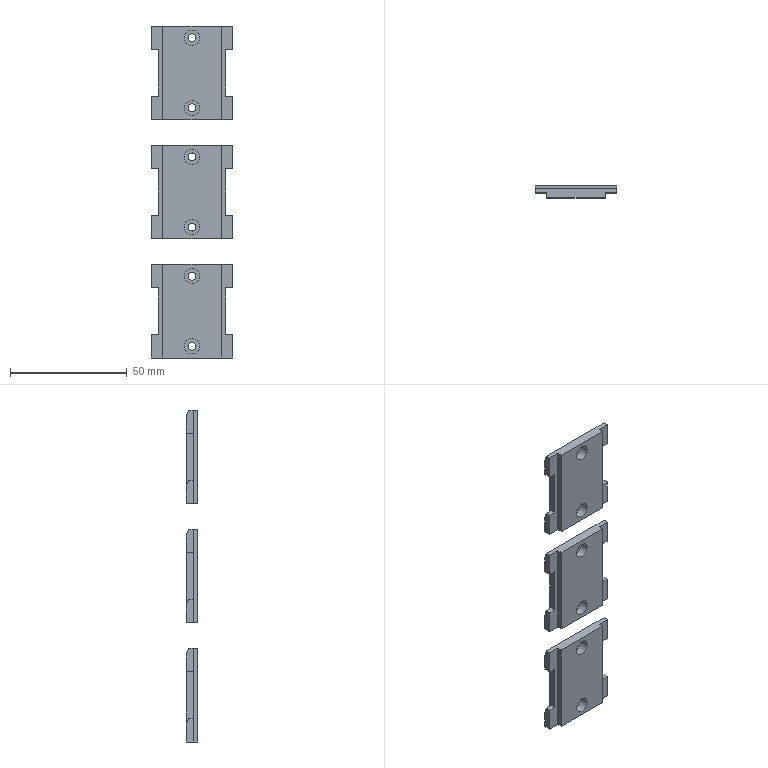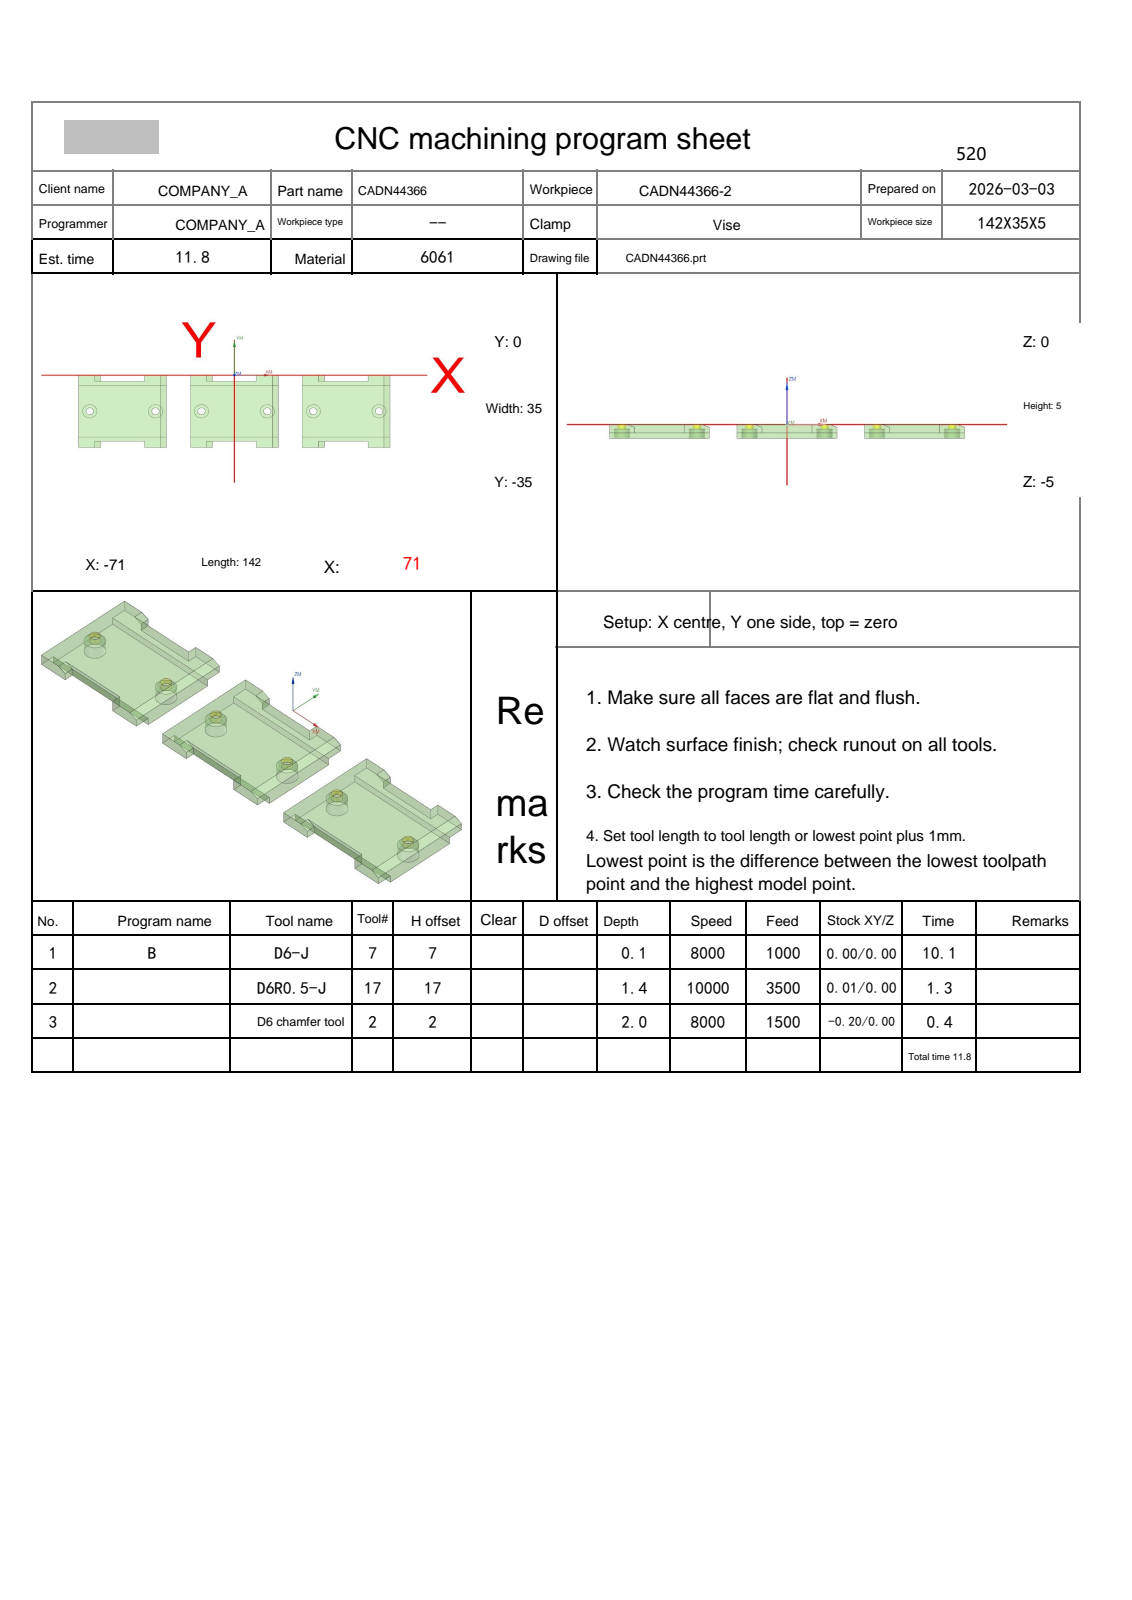NC program | NX | posted by the shop | part box 35 x 5 x 142 mm
Whole program:
%
O0001
(Machine time: 12.44 MIN)
(===Total Tool:3===)
(T7=D6-J    D=6.   R=0.   D-  H07 Z=0.    )
(T17=D6R0.5-J D=6.   R=0.5  D-  H17 Z=-1.41 )
(T2=D6 chamfer tool   D=6.   R=0.   D-  H02 Z=-2.   )
G80 G90 G17 G49 G40
G91 G28 Z0
M01
N1 T07 M06
(D6-J  D=6. R=0. H=07 ce=0.00 di=0.10)
G00 G90 G54 X56.094 Y15. M03 S8000
G43 H07 Z30.
M08
Z4.02
G01 Z2.02 F1000.
X68.094 Y3.
X74. Y-2.906
Y-8.813
X62.188 Y3.
X56.281
X74. Y-14.719
Y-20.625
X50.375 Y3.
X44.469
X74. Y-26.531
Y-32.438
X38.563 Y3.
X32.656
X73.656 Y-38.
X67.75
X26.75 Y3.
X20.844
X61.844 Y-38.
X55.938
X14.938 Y3.
X9.031
X50.031 Y-38.
X44.125
X3.125 Y3.
X-2.781
X38.219 Y-38.
X32.313
X-8.688 Y3.
X-14.594
X26.406 Y-38.
X20.5
X-20.5 Y3.
X-26.406
X14.594 Y-38.
X8.688
X-32.313 Y3.
X-38.219
X2.781 Y-38.
X-3.125
X-44.125 Y3.
X-50.031
X-9.031 Y-38.
X-14.938
X-55.938 Y3.
X-61.844
X-20.844 Y-38.
X-26.75
X-67.75 Y3.
X-73.656
X-32.656 Y-38.
X-38.563
X-74. Y-2.563
Y-8.469
X-44.469 Y-38.
X-50.375
X-74. Y-14.375
Y-20.281
X-56.281 Y-38.
X-62.188
X-74. Y-26.188
Y-32.094
X-68.094 Y-38.
X-56.094 Y-50.
Z4.02
G00 Z5.5
X86. Y-14.906
Z3.54
G01 Z1.54
X74. Y-2.906
X68.094 Y3.
X62.188
X74. Y-8.813
Y-14.719
X56.281 Y3.
X50.375
X74. Y-20.625
Y-26.531
X44.469 Y3.
X38.563
X74. Y-32.438
Y-38.
X73.656
X32.656 Y3.
X26.75
X67.75 Y-38.
X61.844
X20.844 Y3.
X14.938
X55.938 Y-38.
X50.031
X9.031 Y3.
X3.125
X44.125 Y-38.
X38.219
X-2.781 Y3.
X-8.688
X32.313 Y-38.
X26.406
X-14.594 Y3.
X-20.5
X20.5 Y-38.
X14.594
X-26.406 Y3.
X-32.313
X8.688 Y-38.
X2.781
X-38.219 Y3.
X-44.125
X-3.125 Y-38.
X-9.031
X-50.031 Y3.
X-55.938
X-14.938 Y-38.
X-20.844
X-61.844 Y3.
X-67.75
X-26.75 Y-38.
X-32.656
X-73.656 Y3.
X-74.
Y-2.563
X-38.563 Y-38.
X-44.469
X-74. Y-8.469
Y-14.375
X-50.375 Y-38.
X-56.281
X-74. Y-20.281
Y-26.188
X-62.188 Y-38.
X-68.094
X-74. Y-32.094
X-86. Y-20.094
Z3.54
G00 Z5.02
X86. Y-14.906
Z3.06
G01 Z1.06
X74. Y-2.906
X68.094 Y3.
X62.188
X74. Y-8.813
Y-14.719
X56.281 Y3.
X50.375
X74. Y-20.625
Y-26.531
X44.469 Y3.
X38.563
X74. Y-32.438
Y-38.
X73.656
X32.656 Y3.
X26.75
X67.75 Y-38.
X61.844
X20.844 Y3.
X14.938
X55.938 Y-38.
X50.031
X9.031 Y3.
X3.125
X44.125 Y-38.
X38.219
X-2.781 Y3.
X-8.688
X32.313 Y-38.
X26.406
X-14.594 Y3.
X-20.5
X20.5 Y-38.
X14.594
X-26.406 Y3.
X-32.313
X8.688 Y-38.
X2.781
X-38.219 Y3.
X-44.125
X-3.125 Y-38.
X-9.031
X-50.031 Y3.
X-55.938
X-14.938 Y-38.
X-20.844
X-61.844 Y3.
X-67.75
X-26.75 Y-38.
X-32.656
X-73.656 Y3.
X-74.
Y-2.563
X-38.563 Y-38.
X-44.469
X-74. Y-8.469
Y-14.375
X-50.375 Y-38.
X-56.281
X-74. Y-20.281
Y-26.188
X-62.188 Y-38.
X-68.094
X-74. Y-32.094
X-86. Y-20.094
Z3.06
G00 Z4.54
X86. Y-14.906
Z2.58
G01 Z.58
X74. Y-2.906
X68.094 Y3.
X62.188
X74. Y-8.813
Y-14.719
X56.281 Y3.
X50.375
X74. Y-20.625
Y-26.531
X44.469 Y3.
X38.563
X74. Y-32.438
Y-38.
X73.656
X32.656 Y3.
X26.75
X67.75 Y-38.
X61.844
X20.844 Y3.
X14.938
X55.938 Y-38.
X50.031
X9.031 Y3.
X3.125
X44.125 Y-38.
X38.219
X-2.781 Y3.
X-8.688
X32.313 Y-38.
X26.406
X-14.594 Y3.
X-20.5
X20.5 Y-38.
X14.594
X-26.406 Y3.
X-32.313
X8.688 Y-38.
X2.781
X-38.219 Y3.
X-44.125
X-3.125 Y-38.
X-9.031
X-50.031 Y3.
X-55.938
X-14.938 Y-38.
X-20.844
X-61.844 Y3.
X-67.75
X-26.75 Y-38.
X-32.656
X-73.656 Y3.
X-74.
Y-2.563
X-38.563 Y-38.
X-44.469
X-74. Y-8.469
Y-14.375
X-50.375 Y-38.
X-56.281
X-74. Y-20.281
Y-26.188
X-62.188 Y-38.
X-68.094
X-74. Y-32.094
X-86. Y-20.094
Z2.58
G00 Z4.06
X86. Y-14.906
Z2.1
G01 Z.1
X74. Y-2.906
X68.094 Y3.
X62.188
X74. Y-8.813
Y-14.719
X56.281 Y3.
X50.375
X74. Y-20.625
Y-26.531
X44.469 Y3.
X38.563
X74. Y-32.438
Y-38.
X73.656
X32.656 Y3.
X26.75
X67.75 Y-38.
X61.844
X20.844 Y3.
X14.938
X55.938 Y-38.
X50.031
X9.031 Y3.
X3.125
X44.125 Y-38.
X38.219
X-2.781 Y3.
X-8.688
X32.313 Y-38.
X26.406
X-14.594 Y3.
X-20.5
X20.5 Y-38.
X14.594
X-26.406 Y3.
X-32.313
X8.688 Y-38.
X2.781
X-38.219 Y3.
X-44.125
X-3.125 Y-38.
X-9.031
X-50.031 Y3.
X-55.938
X-14.938 Y-38.
X-20.844
X-61.844 Y3.
X-67.75
X-26.75 Y-38.
X-32.656
X-73.656 Y3.
X-74.
Y-2.563
X-38.563 Y-38.
X-44.469
X-74. Y-8.469
Y-14.375
X-50.375 Y-38.
X-56.281
X-74. Y-20.281
Y-26.188
X-62.188 Y-38.
X-68.094
X-74. Y-32.094
X-86. Y-20.094
Z2.1
G00 Z30.
G00 G90 X56.094 Y15. M03 S8000
Z30.
Z2.
G01 Z0.0 F1000.
X68.094 Y3.
X74. Y-2.906
Y-8.813
X62.188 Y3.
X56.281
X74. Y-14.719
Y-20.625
X50.375 Y3.
X44.469
X74. Y-26.531
Y-32.438
X38.563 Y3.
X32.656
X73.656 Y-38.
X67.75
X26.75 Y3.
X20.844
X61.844 Y-38.
X55.938
X14.938 Y3.
X9.031
X50.031 Y-38.
X44.125
X3.125 Y3.
X-2.781
X38.219 Y-38.
X32.313
X-8.688 Y3.
X-14.594
X26.406 Y-38.
X20.5
X-20.5 Y3.
X-26.406
X14.594 Y-38.
X8.688
X-32.313 Y3.
X-38.219
X2.781 Y-38.
X-3.125
X-44.125 Y3.
X-50.031
X-9.031 Y-38.
X-14.938
X-55.938 Y3.
X-61.844
X-20.844 Y-38.
X-26.75
X-67.75 Y3.
X-73.656
X-32.656 Y-38.
X-38.563
X-74. Y-2.563
Y-8.469
X-44.469 Y-38.
X-50.375
X-74. Y-14.375
Y-20.281
X-56.281 Y-38.
X-62.188
X-74. Y-26.188
Y-32.094
X-68.094 Y-38.
X-56.094 Y-50.
Z2.
G00 Z30.
G91 G28 Z0.0
M05
M09
G91 G28 Z0.0
M01
N2 T17 M06
(D6R0.5-J  D=6. R=0.5 H=17 ce=0.01 di=0.00)
G00 G90 G54 X70.938 Y6.124 M03 S10000
G43 H17 Z12.5
M08
Z.466
G01 Z-.034 F3500.
X70.943 Y1.072
X70.945 Y0.0
Y-35.
X70.943 Y-36.072
X70.992 Z-.051
X71.037 Z-.068
X71.039 Y-35.
Y0.0
X71.037 Y1.072
X71.086 Z-.086
X71.131 Z-.103
X71.133 Y0.0
Y-35.
X71.131 Y-36.072
X71.18 Z-.12
X71.225 Z-.137
X71.227 Y-35.
Y0.0
X71.225 Y1.072
X71.274 Z-.154
X71.319 Z-.171
X71.321 Y0.0
Y-35.
X71.319 Y-36.072
X71.368 Z-.188
X71.413 Z-.205
X71.415 Y-35.
Y0.0
X71.413 Y1.072
X71.461 Z-.222
X71.507 Z-.239
X71.508 Y0.0
Y-35.
X71.507 Y-36.072
X71.555 Z-.257
X71.601 Z-.274
X71.602 Y-35.
Y0.0
X71.601 Y1.073
X71.649 Z-.291
X71.695 Z-.308
X71.696 Y0.0
Y-35.
X71.695 Y-36.073
X71.743 Z-.325
X71.789 Z-.342
X71.79 Y-35.
Y0.0
X71.789 Y1.073
X71.837 Z-.359
X71.883 Z-.376
X71.884 Y0.0
Y-35.
X71.883 Y-36.073
X71.931 Z-.393
X71.977 Z-.41
X71.978 Y-35.
Y0.0
X71.977 Y1.073
X72.025 Z-.428
X72.071 Z-.445
X72.072 Y0.0
Y-35.
X72.071 Y-36.073
X72.119 Z-.462
X72.165 Z-.479
X72.166 Y-35.
Y0.0
X72.165 Y1.073
X72.213 Z-.496
X72.259 Z-.513
X72.26 Y0.0
Y-35.
X72.259 Y-36.073
X72.307 Z-.53
X72.353 Z-.547
X72.354 Y-35.
Y0.0
X72.353 Y1.073
X72.401 Z-.564
X72.447 Z-.581
X72.448 Y0.0
Y-35.
X72.447 Y-36.073
X72.495 Z-.599
X72.541 Z-.616
X72.542 Y-35.
Y0.0
X72.541 Y1.073
X72.589 Z-.633
X72.635 Z-.65
X72.636 Y0.0
Y-35.
X72.635 Y-36.073
X72.683 Z-.667
X72.729 Z-.684
X72.73 Y-35.
Y0.0
X72.729 Y1.073
X72.777 Z-.701
X72.823 Z-.718
X72.824 Y0.0
Y-35.
X72.823 Y-36.073
X72.871 Z-.735
X72.917 Z-.752
X72.918 Y-35.
Y0.0
X72.917 Y1.073
X72.965 Z-.77
X73.011 Z-.787
X73.012 Y0.0
Y-35.
X73.011 Y-36.072
X73.059 Z-.804
X73.105 Z-.821
X73.106 Y-35.
Y0.0
X73.105 Y1.072
X73.153 Z-.838
X73.199 Z-.855
X73.2 Y0.0
Y-35.
X73.199 Y-36.072
X73.247 Z-.872
X73.293 Z-.889
X73.294 Y-35.
Y0.0
X73.293 Y1.072
X73.341 Z-.906
X73.387 Z-.923
X73.388 Y0.0
Y-35.
X73.387 Y-36.072
X73.435 Z-.941
X73.481 Z-.958
X73.482 Y-35.
Y0.0
X73.481 Y1.072
X73.529 Z-.975
X73.575 Z-.992
X73.576 Y0.0
Y-35.
X73.575 Y-36.072
X73.623 Z-1.009
X73.669 Z-1.026
X73.67 Y-35.
Y0.0
X73.669 Y1.072
X73.717 Z-1.043
X73.763 Z-1.06
Y-36.072
X73.811 Z-1.077
X73.857 Z-1.094
Y1.072
X73.905 Z-1.112
X73.951 Z-1.129
Y-36.072
X73.999 Z-1.146
X74.044 Z-1.163
X74.045 Y1.071
X74.093 Z-1.18
X74.138 Z-1.197
Y-36.072
X74.187 Z-1.214
X74.232 Y-36.071 Z-1.231
Y1.071
X74.281 Z-1.248
X74.326 Z-1.265
Y-36.071
X74.375 Z-1.283
X74.42 Z-1.3
Y1.071
X74.469 Z-1.317
X74.515 Y1.07 Z-1.334
Y-36.07
X74.562 Y-36.065 Z-1.351
X74.609 Y-36.06 Z-1.368
Y1.06
G00 Z-.905
X77.709 Y-2.377
G01 Z-1.405
X74.712 Y-2.38
Y-5.38
Y-29.62
G00 Z12.5
X19.938 Y6.124
Z.466
G01 Z-.034
X19.944 Y1.072
X19.945 Y0.0
Y-35.
X19.943 Y-36.072
X19.992 Z-.051
X20.037 Z-.068
X20.039 Y-35.
Y0.0
X20.037 Y1.072
X20.086 Z-.086
X20.131 Z-.103
X20.133 Y0.0
Y-35.
X20.131 Y-36.072
X20.18 Z-.12
X20.225 Z-.137
X20.227 Y-35.
Y0.0
X20.225 Y1.072
X20.274 Z-.154
X20.319 Z-.171
X20.321 Y0.0
Y-35.
X20.319 Y-36.072
X20.368 Z-.188
X20.413 Z-.205
X20.415 Y-35.
Y0.0
X20.413 Y1.072
X20.461 Z-.222
X20.507 Z-.239
X20.508 Y0.0
Y-35.
X20.507 Y-36.072
X20.555 Z-.257
X20.601 Z-.274
X20.602 Y-35.
Y0.0
X20.601 Y1.072
X20.649 Y1.073 Z-.291
X20.695 Z-.308
X20.696 Y0.0
Y-35.
X20.695 Y-36.072
X20.743 Y-36.073 Z-.325
X20.789 Z-.342
X20.79 Y-35.
Y0.0
X20.789 Y1.073
X20.837 Z-.359
X20.884 Z-.376
Y0.0
Y-35.
Y-36.073
X20.931 Z-.393
X20.977 Z-.41
X20.978 Y-35.
Y0.0
X20.977 Y1.073
X21.025 Z-.428
X21.071 Z-.445
X21.072 Y0.0
Y-35.
X21.071 Y-36.073
X21.119 Z-.462
X21.165 Z-.479
X21.166 Y-35.
Y0.0
X21.165 Y1.073
X21.213 Z-.496
X21.259 Z-.513
X21.26 Y0.0
Y-35.
X21.259 Y-36.073
X21.307 Z-.53
X21.353 Z-.547
X21.354 Y-35.
Y0.0
X21.353 Y1.073
X21.401 Z-.564
X21.447 Z-.581
X21.448 Y0.0
Y-35.
X21.447 Y-36.073
X21.495 Z-.599
X21.541 Z-.616
X21.542 Y-35.
Y0.0
X21.541 Y1.073
X21.589 Z-.633
X21.635 Z-.65
X21.636 Y0.0
Y-35.
X21.635 Y-36.073
X21.683 Z-.667
X21.729 Z-.684
X21.73 Y-35.
Y0.0
X21.729 Y1.073
X21.777 Z-.701
X21.823 Y1.072 Z-.718
X21.824 Y0.0
Y-35.
X21.823 Y-36.073
X21.871 Z-.735
X21.918 Z-.752
Y-35.
Y0.0
Y1.072
X21.965 Z-.77
X22.011 Z-.787
X22.012 Y0.0
Y-35.
X22.011 Y-36.072
X22.059 Z-.804
X22.105 Z-.821
X22.106 Y-35.
Y0.0
X22.105 Y1.072
X22.153 Z-.838
X22.199 Z-.855
X22.2 Y0.0
Y-35.
X22.199 Y-36.072
X22.247 Z-.872
X22.293 Z-.889
X22.294 Y-35.
Y0.0
X22.293 Y1.072
X22.341 Z-.906
X22.387 Z-.923
X22.388 Y0.0
Y-35.
X22.387 Y-36.072
X22.435 Z-.941
X22.481 Z-.958
X22.482 Y-35.
Y0.0
X22.481 Y1.072
X22.529 Z-.975
X22.575 Z-.992
X22.576 Y0.0
Y-35.
X22.575 Y-36.072
X22.623 Z-1.009
X22.669 Z-1.026
X22.67 Y-35.
Y0.0
X22.669 Y1.072
X22.717 Z-1.043
X22.763 Z-1.06
Y-36.072
X22.811 Z-1.077
X22.857 Z-1.094
Y1.072
X22.905 Z-1.112
X22.951 Z-1.129
Y-36.072
X22.999 Z-1.146
X23.044 Z-1.163
Y1.072
X23.093 Z-1.18
X23.138 Z-1.197
Y-36.071
X23.187 Z-1.214
X23.232 Z-1.231
Y1.071
X23.281 Z-1.248
X23.326 Z-1.265
Y-36.071
X23.375 Z-1.283
X23.42 Z-1.3
Y1.071
X23.469 Z-1.317
X23.514 Z-1.334
Y-36.071
X23.562 Z-1.351
X23.608 Z-1.368
Y1.071
G00 Z-.905
X26.709 Y-2.351
G01 Z-1.405
X23.712 Y-2.354
Y-5.354
Y-29.646
G00 Z12.5
X-31.062 Y6.124
Z.466
G01 Z-.034
X-31.057 Y1.072
X-31.055 Y0.0
Y-35.
X-31.057 Y-36.072
X-31.008 Z-.051
X-30.963 Z-.068
X-30.961 Y-35.
Y0.0
X-30.963 Y1.072
X-30.914 Z-.086
X-30.869 Z-.103
X-30.867 Y0.0
Y-35.
X-30.869 Y-36.072
X-30.82 Z-.12
X-30.775 Z-.137
X-30.773 Y-35.
Y0.0
X-30.775 Y1.072
X-30.726 Z-.154
X-30.681 Z-.171
X-30.679 Y0.0
Y-35.
X-30.681 Y-36.072
X-30.632 Z-.188
X-30.587 Z-.205
X-30.585 Y-35.
Y0.0
X-30.587 Y1.072
X-30.539 Z-.222
X-30.493 Z-.239
X-30.492 Y0.0
Y-35.
X-30.493 Y-36.072
X-30.445 Z-.257
X-30.399 Z-.274
X-30.398 Y-35.
Y0.0
X-30.399 Y1.072
X-30.351 Y1.073 Z-.291
X-30.305 Z-.308
X-30.304 Y0.0
Y-35.
X-30.305 Y-36.072
X-30.257 Y-36.073 Z-.325
X-30.211 Z-.342
X-30.21 Y-35.
Y0.0
X-30.211 Y1.073
X-30.163 Z-.359
X-30.116 Z-.376
Y0.0
Y-35.
Y-36.073
X-30.069 Z-.393
X-30.023 Z-.41
X-30.022 Y-35.
Y0.0
X-30.023 Y1.073
X-29.975 Z-.428
X-29.929 Z-.445
X-29.928 Y0.0
Y-35.
X-29.929 Y-36.073
X-29.881 Z-.462
X-29.835 Z-.479
X-29.834 Y-35.
Y0.0
X-29.835 Y1.073
X-29.787 Z-.496
X-29.741 Z-.513
X-29.74 Y0.0
Y-35.
X-29.741 Y-36.073
X-29.693 Z-.53
X-29.647 Z-.547
X-29.646 Y-35.
Y0.0
X-29.647 Y1.073
X-29.599 Z-.564
X-29.553 Z-.581
X-29.552 Y0.0
Y-35.
X-29.553 Y-36.073
X-29.505 Z-.599
X-29.459 Z-.616
X-29.458 Y-35.
Y0.0
X-29.459 Y1.073
X-29.411 Z-.633
X-29.365 Z-.65
X-29.364 Y0.0
Y-35.
X-29.365 Y-36.073
X-29.317 Z-.667
X-29.271 Z-.684
X-29.27 Y-35.
Y0.0
X-29.271 Y1.073
X-29.223 Z-.701
X-29.177 Y1.072 Z-.718
X-29.176 Y0.0
Y-35.
X-29.177 Y-36.073
X-29.129 Z-.735
X-29.082 Z-.752
Y-35.
Y0.0
Y1.072
X-29.035 Z-.77
X-28.989 Z-.787
X-28.988 Y0.0
Y-35.
X-28.989 Y-36.072
X-28.941 Z-.804
X-28.895 Z-.821
X-28.894 Y-35.
Y0.0
X-28.895 Y1.072
X-28.847 Z-.838
X-28.801 Z-.855
X-28.8 Y0.0
Y-35.
X-28.801 Y-36.072
X-28.753 Z-.872
X-28.707 Z-.889
X-28.706 Y-35.
Y0.0
X-28.707 Y1.072
X-28.659 Z-.906
X-28.613 Z-.923
X-28.612 Y0.0
Y-35.
X-28.613 Y-36.072
X-28.565 Z-.941
X-28.519 Z-.958
X-28.518 Y-35.
Y0.0
X-28.519 Y1.072
X-28.471 Z-.975
X-28.425 Z-.992
X-28.424 Y0.0
Y-35.
X-28.425 Y-36.072
X-28.377 Z-1.009
X-28.331 Z-1.026
X-28.33 Y-35.
Y0.0
X-28.331 Y1.072
X-28.283 Z-1.043
X-28.237 Z-1.06
Y-36.072
X-28.189 Z-1.077
X-28.143 Z-1.094
Y1.072
X-28.095 Z-1.112
X-28.049 Z-1.129
Y-36.072
X-28.001 Z-1.146
X-27.956 Z-1.163
Y1.072
X-27.907 Z-1.18
X-27.862 Z-1.197
Y-36.071
X-27.813 Z-1.214
X-27.768 Z-1.231
Y1.071
X-27.719 Z-1.248
X-27.674 Z-1.265
Y-36.071
X-27.625 Z-1.283
X-27.58 Z-1.3
Y1.071
X-27.531 Z-1.317
X-27.486 Z-1.334
Y-36.071
X-27.438 Z-1.351
X-27.392 Z-1.368
Y1.071
G00 Z-.905
X-24.291 Y-2.351
G01 Z-1.405
X-27.288 Y-2.354
Y-5.354
Y-29.646
G00 Z12.5
G91 G28 Z0.0
M05
M09
G91 G28 Z0.0
M01
N3 T02 M06
(D6 chamfer tool  D=6. R=0. H=02 ce=-0.20 di=0.00)
G00 G90 G54 X39.243 Y-35.8 M03 S7000
G43 H02 Z30.
M08
Z2.5
G01 X31.122 Z-.456 F1500.
X30.923 Y-35.764 Z-.529
X30.735 Y-35.689 Z-.603
X30.566 Y-35.577 Z-.677
X30.423 Y-35.434 Z-.751
X30.311 Y-35.265 Z-.824
X30.236 Y-35.077 Z-.898
X30.2 Y-34.878 Z-.972
Y-34.8 Z-1.
Y-.2
G02 X31.2 Y.8 I1. J0.0
G01 X40.8
G02 X41.8 Y-.2 I0.0 J-1.
G01 Y-2.2
X60.2
Y-.2
G02 X61.2 Y.8 I1. J0.0
G01 X70.8
G02 X71.8 Y-.2 I0.0 J-1.
G01 Y-34.8
G02 X70.8 Y-35.8 I-1. J0.0
G01 X61.2
G02 X60.2 Y-34.8 I0.0 J1.
G01 Y-32.8
X41.8
Y-34.8
G02 X40.8 Y-35.8 I-1. J0.0
G01 X31.2
G02 X30.2 Y-34.8 I0.0 J1.
G01 Y-34.3
Z1.5
G00 Z30.
X-11.757 Y-35.8
Z2.5
G01 X-19.878 Z-.456
X-20.077 Y-35.764 Z-.529
X-20.265 Y-35.689 Z-.603
X-20.434 Y-35.577 Z-.677
X-20.577 Y-35.434 Z-.751
X-20.689 Y-35.265 Z-.824
X-20.764 Y-35.077 Z-.898
X-20.8 Y-34.878 Z-.972
Y-34.8 Z-1.
Y-.2
G02 X-19.8 Y.8 I1. J0.0
G01 X-10.2
G02 X-9.2 Y-.2 I0.0 J-1.
G01 Y-2.2
X9.2
Y-.2
G02 X10.2 Y.8 I1. J0.0
G01 X19.8
G02 X20.8 Y-.2 I0.0 J-1.
G01 Y-34.8
G02 X19.8 Y-35.8 I-1. J0.0
G01 X10.2
G02 X9.2 Y-34.8 I0.0 J1.
G01 Y-32.8
X-9.2
Y-34.8
G02 X-10.2 Y-35.8 I-1. J0.0
G01 X-19.8
G02 X-20.8 Y-34.8 I0.0 J1.
G01 Y-34.3
Z1.5
G00 Z30.
X-62.757 Y-35.8
Z2.5
G01 X-70.878 Z-.456
X-71.077 Y-35.764 Z-.529
X-71.265 Y-35.689 Z-.603
X-71.434 Y-35.577 Z-.677
X-71.577 Y-35.434 Z-.751
X-71.689 Y-35.265 Z-.824
X-71.764 Y-35.077 Z-.898
X-71.8 Y-34.878 Z-.972
Y-34.8 Z-1.
Y-.2
G02 X-70.8 Y.8 I1. J0.0
G01 X-61.2
G02 X-60.2 Y-.2 I0.0 J-1.
G01 Y-2.2
X-41.8
Y-.2
G02 X-40.8 Y.8 I1. J0.0
G01 X-31.2
G02 X-30.2 Y-.2 I0.0 J-1.
G01 Y-34.8
G02 X-31.2 Y-35.8 I-1. J0.0
G01 X-40.8
G02 X-41.8 Y-34.8 I0.0 J1.
G01 Y-32.8
X-60.2
Y-34.8
G02 X-61.2 Y-35.8 I-1. J0.0
G01 X-70.8
G02 X-71.8 Y-34.8 I0.0 J1.
G01 Y-34.3
Z1.5
G00 Z30.
G00 G90 X66. Y-17.5 M03 S8000
Z30.
G98 G81 X66. Y-17.5 Z-2. R3. F1000.
X36.
X15.
X-15.
X-36.
X-66.
G80
G00 Z30.
M05
M09
G91 G28 Z0.0
G91 G28 Y0.0
M30
%